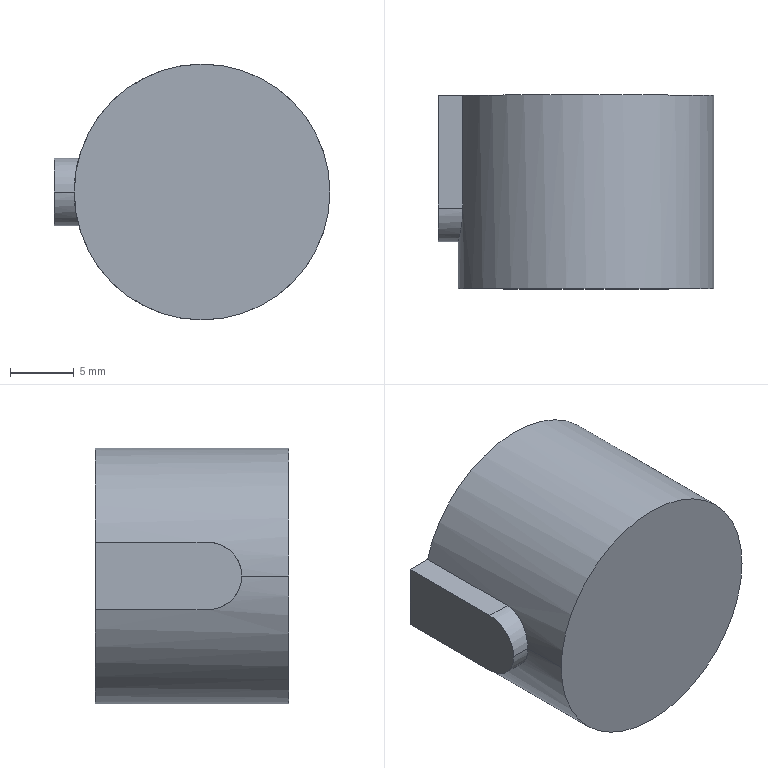Part | SolidWorks | features BaseBody 1 | 1 solid | 9 faces | box 21.648 x 15.198 x 20.064 mm | volume 4903 mm3 | plane 5 | cylinder 4 | commonest cylinder face diameters 5.28 x2 20.064 x2
STEP:
#1=CARTESIAN_POINT('',(-2122.918,1097.894,-1577.624));
#2=VERTEX_POINT('',#1);
#3=CARTESIAN_POINT('',(-2122.918,1082.696,-1577.624));
#4=VERTEX_POINT('',#3);
#5=CARTESIAN_POINT('',(-2122.918,1097.894,-1577.624));
#6=DIRECTION('',(0.,-1.,0.));
#7=VECTOR('',#6,1000.);
#8=LINE('',#5,#7);
#9=EDGE_CURVE('',#2,#4,#8,.T.);
#10=ORIENTED_EDGE('',*,*,#9,.F.);
#11=CARTESIAN_POINT('',(-2142.628,1097.894,-1574.984));
#12=VERTEX_POINT('',#11);
#13=CARTESIAN_POINT('',(-2132.95,1097.894,-1577.624));
#14=DIRECTION('',(0.,-1.,0.));
#15=DIRECTION('',(1.,0.,0.));
#16=AXIS2_PLACEMENT_3D('',#13,#14,#15);
#17=CIRCLE('',#16,10.032);
#18=EDGE_CURVE('',#2,#12,#17,.T.);
#19=ORIENTED_EDGE('',*,*,#18,.T.);
#20=CARTESIAN_POINT('',(-2142.628,1089.032,-1574.984));
#21=VERTEX_POINT('',#20);
#22=CARTESIAN_POINT('',(-2142.628,1089.032,-1574.984));
#23=DIRECTION('',(0.,1.,0.));
#24=VECTOR('',#23,1000.);
#25=LINE('',#22,#24);
#26=EDGE_CURVE('',#21,#12,#25,.T.);
#27=ORIENTED_EDGE('',*,*,#26,.F.);
#28=CARTESIAN_POINT('',(-2142.982,1086.392,-1577.624));
#29=VERTEX_POINT('',#28);
#30=CARTESIAN_POINT('',(-2142.982,1086.392,-1577.624));
#31=CARTESIAN_POINT('',(-2142.982,1086.392,-1577.461));
#32=CARTESIAN_POINT('',(-2142.978,1086.407,-1577.293));
#33=CARTESIAN_POINT('',(-2142.965,1086.456,-1577.038));
#34=CARTESIAN_POINT('',(-2142.959,1086.477,-1576.952));
#35=CARTESIAN_POINT('',(-2142.95,1086.516,-1576.824));
#36=CARTESIAN_POINT('',(-2142.945,1086.537,-1576.761));
#37=CARTESIAN_POINT('',(-2142.938,1086.564,-1576.686));
#38=CARTESIAN_POINT('',(-2142.935,1086.577,-1576.654));
#39=CARTESIAN_POINT('',(-2142.933,1086.585,-1576.633));
#40=CARTESIAN_POINT('',(-2142.931,1086.59,-1576.621));
#41=CARTESIAN_POINT('',(-2142.923,1086.624,-1576.54));
#42=CARTESIAN_POINT('',(-2142.915,1086.659,-1576.465));
#43=CARTESIAN_POINT('',(-2142.9,1086.719,-1576.35));
#44=CARTESIAN_POINT('',(-2142.895,1086.741,-1576.312));
#45=CARTESIAN_POINT('',(-2142.888,1086.776,-1576.254));
#46=CARTESIAN_POINT('',(-2142.884,1086.793,-1576.224));
#47=CARTESIAN_POINT('',(-2142.879,1086.815,-1576.19));
#48=CARTESIAN_POINT('',(-2142.877,1086.825,-1576.176));
#49=CARTESIAN_POINT('',(-2142.875,1086.831,-1576.166));
#50=CARTESIAN_POINT('',(-2142.874,1086.836,-1576.159));
#51=CARTESIAN_POINT('',(-2142.866,1086.871,-1576.106));
#52=CARTESIAN_POINT('',(-2142.857,1086.914,-1576.046));
#53=CARTESIAN_POINT('',(-2142.84,1086.994,-1575.945));
#54=CARTESIAN_POINT('',(-2142.834,1087.024,-1575.91));
#55=CARTESIAN_POINT('',(-2142.824,1087.073,-1575.854));
#56=CARTESIAN_POINT('',(-2142.821,1087.09,-1575.835));
#57=CARTESIAN_POINT('',(-2142.814,1087.127,-1575.797));
#58=CARTESIAN_POINT('',(-2142.81,1087.144,-1575.778));
#59=CARTESIAN_POINT('',(-2142.791,1087.249,-1575.674));
#60=CARTESIAN_POINT('',(-2142.777,1087.326,-1575.608));
#61=CARTESIAN_POINT('',(-2142.76,1087.427,-1575.528));
#62=CARTESIAN_POINT('',(-2142.755,1087.459,-1575.504));
#63=CARTESIAN_POINT('',(-2142.748,1087.501,-1575.473));
#64=CARTESIAN_POINT('',(-2142.745,1087.522,-1575.459));
#65=CARTESIAN_POINT('',(-2142.742,1087.543,-1575.444));
#66=CARTESIAN_POINT('',(-2142.74,1087.554,-1575.437));
#67=CARTESIAN_POINT('',(-2142.74,1087.558,-1575.434));
#68=CARTESIAN_POINT('',(-2142.739,1087.561,-1575.432));
#69=CARTESIAN_POINT('',(-2142.739,1087.561,-1575.432));
#70=CARTESIAN_POINT('',(-2142.727,1087.643,-1575.377));
#71=CARTESIAN_POINT('',(-2142.716,1087.721,-1575.331));
#72=CARTESIAN_POINT('',(-2142.702,1087.835,-1575.271));
#73=CARTESIAN_POINT('',(-2142.697,1087.873,-1575.252));
#74=CARTESIAN_POINT('',(-2142.691,1087.929,-1575.226));
#75=CARTESIAN_POINT('',(-2142.688,1087.956,-1575.213));
#76=CARTESIAN_POINT('',(-2142.685,1087.984,-1575.201));
#77=CARTESIAN_POINT('',(-2142.683,1088.002,-1575.194));
#78=CARTESIAN_POINT('',(-2142.682,1088.009,-1575.191));
#79=CARTESIAN_POINT('',(-2142.646,1088.36,-1575.045));
#80=CARTESIAN_POINT('',(-2142.628,1088.707,-1574.984));
#81=CARTESIAN_POINT('',(-2142.628,1089.032,-1574.984));
#82=B_SPLINE_CURVE_WITH_KNOTS('',3,(#30,#31,#32,#33,#34,#35,#36,#37,#38,#39,#40,#41,#42,#43,#44,#45,#46,#47,#48,#49,#50,#51,#52,#53,#54,#55,#56,#57,#58,#59,#60,#61,#62,#63,#64,#65,#66,#67,#68,#69,#70,#71,#72,#73,#74,#75,#76,#77,#78,#79,#80,#81),.UNSPECIFIED.,.F.,.F.,(4,2,2,1,1,2,2,2,2,1,1,2,2,2,2,2,2,2,2,1,1,1,2,2,2,2,1,2,2,4),(0.,0.125,0.1875,0.2187,0.2344,0.2422,0.25,0.3125,0.3437,0.3594,0.3672,0.3711,0.375,0.4375,0.4687,0.4844,0.5,0.5625,0.5937,0.6094,0.6172,0.6211,0.623,0.625,0.6875,0.7187,0.7344,0.7422,0.75,1.),.UNSPECIFIED.);
#83=EDGE_CURVE('',#29,#21,#82,.T.);
#84=ORIENTED_EDGE('',*,*,#83,.F.);
#85=CARTESIAN_POINT('',(-2142.982,1082.696,-1577.624));
#86=VERTEX_POINT('',#85);
#87=CARTESIAN_POINT('',(-2142.982,1086.392,-1577.624));
#88=DIRECTION('',(0.,-1.,0.));
#89=VECTOR('',#88,1000.);
#90=LINE('',#87,#89);
#91=EDGE_CURVE('',#29,#86,#90,.T.);
#92=ORIENTED_EDGE('',*,*,#91,.T.);
#93=CARTESIAN_POINT('',(-2132.95,1082.696,-1577.624));
#94=DIRECTION('',(0.,-1.,0.));
#95=DIRECTION('',(1.,0.,0.));
#96=AXIS2_PLACEMENT_3D('',#93,#94,#95);
#97=CIRCLE('',#96,10.032);
#98=EDGE_CURVE('',#4,#86,#97,.T.);
#99=ORIENTED_EDGE('',*,*,#98,.F.);
#100=EDGE_LOOP('',(#10,#19,#27,#84,#92,#99));
#101=FACE_OUTER_BOUND('',#100,.T.);
#102=CARTESIAN_POINT('',(-2132.95,1080.69,-1577.624));
#103=DIRECTION('',(0.,-1.,0.));
#104=DIRECTION('',(0.9962,0.,-0.08716));
#105=AXIS2_PLACEMENT_3D('',#102,#103,#104);
#106=CYLINDRICAL_SURFACE('',#105,10.032);
#107=ADVANCED_FACE('',(#101),#106,.T.);
#108=CARTESIAN_POINT('',(-2144.566,1097.894,-1580.264));
#109=VERTEX_POINT('',#108);
#110=CARTESIAN_POINT('',(-2144.566,1097.894,-1574.984));
#111=VERTEX_POINT('',#110);
#112=CARTESIAN_POINT('',(-2144.566,1097.894,-1580.264));
#113=DIRECTION('',(0.,0.,1.));
#114=VECTOR('',#113,1000.);
#115=LINE('',#112,#114);
#116=EDGE_CURVE('',#109,#111,#115,.T.);
#117=ORIENTED_EDGE('',*,*,#116,.F.);
#118=CARTESIAN_POINT('',(-2144.566,1089.032,-1580.264));
#119=VERTEX_POINT('',#118);
#120=CARTESIAN_POINT('',(-2144.566,1097.894,-1580.264));
#121=DIRECTION('',(0.,-1.,0.));
#122=VECTOR('',#121,1000.);
#123=LINE('',#120,#122);
#124=EDGE_CURVE('',#109,#119,#123,.T.);
#125=ORIENTED_EDGE('',*,*,#124,.T.);
#126=CARTESIAN_POINT('',(-2144.566,1086.392,-1577.624));
#127=VERTEX_POINT('',#126);
#128=CARTESIAN_POINT('',(-2144.566,1089.032,-1577.624));
#129=DIRECTION('',(-1.,0.,0.));
#130=DIRECTION('',(0.,0.,-1.));
#131=AXIS2_PLACEMENT_3D('',#128,#129,#130);
#132=CIRCLE('',#131,2.64);
#133=EDGE_CURVE('',#119,#127,#132,.T.);
#134=ORIENTED_EDGE('',*,*,#133,.T.);
#135=CARTESIAN_POINT('',(-2144.566,1089.032,-1574.984));
#136=VERTEX_POINT('',#135);
#137=CARTESIAN_POINT('',(-2144.566,1089.032,-1577.624));
#138=DIRECTION('',(-1.,0.,0.));
#139=DIRECTION('',(0.,-1.,0.));
#140=AXIS2_PLACEMENT_3D('',#137,#138,#139);
#141=CIRCLE('',#140,2.64);
#142=EDGE_CURVE('',#127,#136,#141,.T.);
#143=ORIENTED_EDGE('',*,*,#142,.T.);
#144=CARTESIAN_POINT('',(-2144.566,1089.032,-1574.984));
#145=DIRECTION('',(0.,1.,0.));
#146=VECTOR('',#145,1000.);
#147=LINE('',#144,#146);
#148=EDGE_CURVE('',#136,#111,#147,.T.);
#149=ORIENTED_EDGE('',*,*,#148,.T.);
#150=EDGE_LOOP('',(#117,#125,#134,#143,#149));
#151=FACE_OUTER_BOUND('',#150,.T.);
#152=CARTESIAN_POINT('',(-2144.566,1084.729,-1573.321));
#153=DIRECTION('',(-1.,0.,0.));
#154=DIRECTION('',(0.,0.,1.));
#155=AXIS2_PLACEMENT_3D('',#152,#153,#154);
#156=PLANE('',#155);
#157=ADVANCED_FACE('',(#151),#156,.T.);
#158=ORIENTED_EDGE('',*,*,#142,.F.);
#159=CARTESIAN_POINT('',(-2144.566,1086.392,-1577.624));
#160=DIRECTION('',(1.,0.,0.));
#161=VECTOR('',#160,1000.);
#162=LINE('',#159,#161);
#163=EDGE_CURVE('',#127,#29,#162,.T.);
#164=ORIENTED_EDGE('',*,*,#163,.T.);
#165=ORIENTED_EDGE('',*,*,#83,.T.);
#166=CARTESIAN_POINT('',(-2142.628,1089.032,-1574.984));
#167=DIRECTION('',(-1.,-0.000000001,0.));
#168=VECTOR('',#167,1000.);
#169=LINE('',#166,#168);
#170=EDGE_CURVE('',#21,#136,#169,.T.);
#171=ORIENTED_EDGE('',*,*,#170,.T.);
#172=EDGE_LOOP('',(#158,#164,#165,#171));
#173=FACE_OUTER_BOUND('',#172,.T.);
#174=CARTESIAN_POINT('',(-2142.531,1089.032,-1577.624));
#175=DIRECTION('',(1.,0.,0.));
#176=DIRECTION('',(0.,0.08716,0.9962));
#177=AXIS2_PLACEMENT_3D('',#174,#175,#176);
#178=CYLINDRICAL_SURFACE('',#177,2.64);
#179=ADVANCED_FACE('',(#173),#178,.T.);
#180=ORIENTED_EDGE('',*,*,#26,.T.);
#181=CARTESIAN_POINT('',(-2144.566,1097.894,-1574.984));
#182=DIRECTION('',(1.,0.,0.));
#183=VECTOR('',#182,1000.);
#184=LINE('',#181,#183);
#185=EDGE_CURVE('',#111,#12,#184,.T.);
#186=ORIENTED_EDGE('',*,*,#185,.F.);
#187=ORIENTED_EDGE('',*,*,#148,.F.);
#188=ORIENTED_EDGE('',*,*,#170,.F.);
#189=EDGE_LOOP('',(#180,#186,#187,#188));
#190=FACE_OUTER_BOUND('',#189,.T.);
#191=CARTESIAN_POINT('',(-2141.229,1118.415,-1574.984));
#192=DIRECTION('',(0.,0.,1.));
#193=DIRECTION('',(1.,0.,0.));
#194=AXIS2_PLACEMENT_3D('',#191,#192,#193);
#195=PLANE('',#194);
#196=ADVANCED_FACE('',(#190),#195,.T.);
#197=CARTESIAN_POINT('',(-2142.628,1097.894,-1580.264));
#198=VERTEX_POINT('',#197);
#199=CARTESIAN_POINT('',(-2142.628,1097.894,-1580.264));
#200=DIRECTION('',(-1.,0.,0.));
#201=VECTOR('',#200,1000.);
#202=LINE('',#199,#201);
#203=EDGE_CURVE('',#198,#109,#202,.T.);
#204=ORIENTED_EDGE('',*,*,#203,.F.);
#205=CARTESIAN_POINT('',(-2142.628,1089.032,-1580.264));
#206=VERTEX_POINT('',#205);
#207=CARTESIAN_POINT('',(-2142.628,1097.894,-1580.264));
#208=DIRECTION('',(0.,-1.,0.));
#209=VECTOR('',#208,1000.);
#210=LINE('',#207,#209);
#211=EDGE_CURVE('',#198,#206,#210,.T.);
#212=ORIENTED_EDGE('',*,*,#211,.T.);
#213=CARTESIAN_POINT('',(-2142.628,1089.032,-1580.264));
#214=DIRECTION('',(-1.,0.,0.));
#215=VECTOR('',#214,1000.);
#216=LINE('',#213,#215);
#217=EDGE_CURVE('',#206,#119,#216,.T.);
#218=ORIENTED_EDGE('',*,*,#217,.T.);
#219=ORIENTED_EDGE('',*,*,#124,.F.);
#220=EDGE_LOOP('',(#204,#212,#218,#219));
#221=FACE_OUTER_BOUND('',#220,.T.);
#222=CARTESIAN_POINT('',(-2145.965,1118.415,-1580.264));
#223=DIRECTION('',(0.,0.,-1.));
#224=DIRECTION('',(0.,-1.,0.));
#225=AXIS2_PLACEMENT_3D('',#222,#223,#224);
#226=PLANE('',#225);
#227=ADVANCED_FACE('',(#221),#226,.T.);
#228=CARTESIAN_POINT('',(-2132.95,1082.696,-1577.624));
#229=DIRECTION('',(0.,-1.,0.));
#230=DIRECTION('',(-1.,0.,0.));
#231=AXIS2_PLACEMENT_3D('',#228,#229,#230);
#232=CIRCLE('',#231,10.032);
#233=EDGE_CURVE('',#86,#4,#232,.T.);
#234=ORIENTED_EDGE('',*,*,#233,.T.);
#235=ORIENTED_EDGE('',*,*,#98,.T.);
#236=EDGE_LOOP('',(#234,#235));
#237=FACE_OUTER_BOUND('',#236,.T.);
#238=CARTESIAN_POINT('',(-2143.985,1082.696,-1588.66));
#239=DIRECTION('',(0.,-1.,0.));
#240=DIRECTION('',(0.,0.,-1.));
#241=AXIS2_PLACEMENT_3D('',#238,#239,#240);
#242=PLANE('',#241);
#243=ADVANCED_FACE('',(#237),#242,.T.);
#244=ORIENTED_EDGE('',*,*,#163,.F.);
#245=ORIENTED_EDGE('',*,*,#133,.F.);
#246=ORIENTED_EDGE('',*,*,#217,.F.);
#247=CARTESIAN_POINT('',(-2142.628,1089.032,-1580.264));
#248=CARTESIAN_POINT('',(-2142.628,1088.87,-1580.264));
#249=CARTESIAN_POINT('',(-2142.632,1088.702,-1580.249));
#250=CARTESIAN_POINT('',(-2142.646,1088.447,-1580.2));
#251=CARTESIAN_POINT('',(-2142.651,1088.361,-1580.179));
#252=CARTESIAN_POINT('',(-2142.661,1088.233,-1580.141));
#253=CARTESIAN_POINT('',(-2142.666,1088.169,-1580.12));
#254=CARTESIAN_POINT('',(-2142.673,1088.094,-1580.092));
#255=CARTESIAN_POINT('',(-2142.677,1088.062,-1580.08));
#256=CARTESIAN_POINT('',(-2142.679,1088.041,-1580.071));
#257=CARTESIAN_POINT('',(-2142.68,1088.029,-1580.066));
#258=CARTESIAN_POINT('',(-2142.688,1087.948,-1580.033));
#259=CARTESIAN_POINT('',(-2142.697,1087.874,-1579.998));
#260=CARTESIAN_POINT('',(-2142.711,1087.759,-1579.938));
#261=CARTESIAN_POINT('',(-2142.716,1087.72,-1579.916));
#262=CARTESIAN_POINT('',(-2142.725,1087.662,-1579.881));
#263=CARTESIAN_POINT('',(-2142.729,1087.633,-1579.863));
#264=CARTESIAN_POINT('',(-2142.734,1087.598,-1579.841));
#265=CARTESIAN_POINT('',(-2142.736,1087.581,-1579.83));
#266=CARTESIAN_POINT('',(-2142.737,1087.574,-1579.825));
#267=CARTESIAN_POINT('',(-2142.738,1087.569,-1579.822));
#268=CARTESIAN_POINT('',(-2142.739,1087.565,-1579.819));
#269=CARTESIAN_POINT('',(-2142.746,1087.519,-1579.788));
#270=CARTESIAN_POINT('',(-2142.755,1087.461,-1579.748));
#271=CARTESIAN_POINT('',(-2142.771,1087.36,-1579.668));
#272=CARTESIAN_POINT('',(-2142.778,1087.324,-1579.638));
#273=CARTESIAN_POINT('',(-2142.788,1087.266,-1579.587));
#274=CARTESIAN_POINT('',(-2142.791,1087.247,-1579.57));
#275=CARTESIAN_POINT('',(-2142.799,1087.207,-1579.532));
#276=CARTESIAN_POINT('',(-2142.803,1087.185,-1579.511));
#277=CARTESIAN_POINT('',(-2142.821,1087.086,-1579.412));
#278=CARTESIAN_POINT('',(-2142.835,1087.021,-1579.337));
#279=CARTESIAN_POINT('',(-2142.851,1086.941,-1579.236));
#280=CARTESIAN_POINT('',(-2142.856,1086.917,-1579.204));
#281=CARTESIAN_POINT('',(-2142.863,1086.884,-1579.16));
#282=CARTESIAN_POINT('',(-2142.867,1086.869,-1579.139));
#283=CARTESIAN_POINT('',(-2142.87,1086.853,-1579.115));
#284=CARTESIAN_POINT('',(-2142.872,1086.846,-1579.105));
#285=CARTESIAN_POINT('',(-2142.873,1086.842,-1579.099));
#286=CARTESIAN_POINT('',(-2142.873,1086.841,-1579.098));
#287=CARTESIAN_POINT('',(-2142.885,1086.786,-1579.015));
#288=CARTESIAN_POINT('',(-2142.896,1086.74,-1578.937));
#289=CARTESIAN_POINT('',(-2142.91,1086.679,-1578.822));
#290=CARTESIAN_POINT('',(-2142.914,1086.66,-1578.784));
#291=CARTESIAN_POINT('',(-2142.921,1086.634,-1578.728));
#292=CARTESIAN_POINT('',(-2142.924,1086.621,-1578.701));
#293=CARTESIAN_POINT('',(-2142.927,1086.609,-1578.673));
#294=CARTESIAN_POINT('',(-2142.929,1086.601,-1578.655));
#295=CARTESIAN_POINT('',(-2142.929,1086.598,-1578.647));
#296=CARTESIAN_POINT('',(-2142.965,1086.453,-1578.299));
#297=CARTESIAN_POINT('',(-2142.982,1086.392,-1577.951));
#298=CARTESIAN_POINT('',(-2142.982,1086.392,-1577.624));
#299=B_SPLINE_CURVE_WITH_KNOTS('',3,(#247,#248,#249,#250,#251,#252,#253,#254,#255,#256,#257,#258,#259,#260,#261,#262,#263,#264,#265,#266,#267,#268,#269,#270,#271,#272,#273,#274,#275,#276,#277,#278,#279,#280,#281,#282,#283,#284,#285,#286,#287,#288,#289,#290,#291,#292,#293,#294,#295,#296,#297,#298),.UNSPECIFIED.,.F.,.F.,(4,2,2,1,1,2,2,2,2,1,1,1,2,2,2,2,2,2,2,2,1,1,2,2,2,2,1,2,2,4),(0.,0.125,0.1875,0.2187,0.2344,0.2422,0.25,0.3125,0.3437,0.3594,0.3672,0.3711,0.373,0.375,0.4375,0.4687,0.4844,0.5,0.5625,0.5937,0.6094,0.6172,0.6211,0.625,0.6875,0.7187,0.7344,0.7422,0.75,1.),.UNSPECIFIED.);
#300=EDGE_CURVE('',#206,#29,#299,.T.);
#301=ORIENTED_EDGE('',*,*,#300,.T.);
#302=EDGE_LOOP('',(#244,#245,#246,#301));
#303=FACE_OUTER_BOUND('',#302,.T.);
#304=CARTESIAN_POINT('',(-2142.531,1089.032,-1577.624));
#305=DIRECTION('',(1.,0.,0.));
#306=DIRECTION('',(0.,-0.9962,0.08716));
#307=AXIS2_PLACEMENT_3D('',#304,#305,#306);
#308=CYLINDRICAL_SURFACE('',#307,2.64);
#309=ADVANCED_FACE('',(#303),#308,.T.);
#310=CARTESIAN_POINT('',(-2132.95,1097.894,-1577.624));
#311=DIRECTION('',(0.,-1.,0.));
#312=DIRECTION('',(-0.9648,0.,-0.2632));
#313=AXIS2_PLACEMENT_3D('',#310,#311,#312);
#314=CIRCLE('',#313,10.032);
#315=EDGE_CURVE('',#198,#2,#314,.T.);
#316=ORIENTED_EDGE('',*,*,#315,.T.);
#317=ORIENTED_EDGE('',*,*,#9,.T.);
#318=ORIENTED_EDGE('',*,*,#233,.F.);
#319=ORIENTED_EDGE('',*,*,#91,.F.);
#320=ORIENTED_EDGE('',*,*,#300,.F.);
#321=ORIENTED_EDGE('',*,*,#211,.F.);
#322=EDGE_LOOP('',(#316,#317,#318,#319,#320,#321));
#323=FACE_OUTER_BOUND('',#322,.T.);
#324=CARTESIAN_POINT('',(-2132.95,1080.69,-1577.624));
#325=DIRECTION('',(0.,-1.,0.));
#326=DIRECTION('',(-0.9962,0.,0.08716));
#327=AXIS2_PLACEMENT_3D('',#324,#325,#326);
#328=CYLINDRICAL_SURFACE('',#327,10.032);
#329=ADVANCED_FACE('',(#323),#328,.T.);
#330=ORIENTED_EDGE('',*,*,#315,.F.);
#331=ORIENTED_EDGE('',*,*,#203,.T.);
#332=ORIENTED_EDGE('',*,*,#116,.T.);
#333=ORIENTED_EDGE('',*,*,#185,.T.);
#334=ORIENTED_EDGE('',*,*,#18,.F.);
#335=EDGE_LOOP('',(#330,#331,#332,#333,#334));
#336=FACE_OUTER_BOUND('',#335,.T.);
#337=CARTESIAN_POINT('',(-2200.45,1097.894,-1510.124));
#338=DIRECTION('',(0.,1.,0.));
#339=DIRECTION('',(1.,0.,0.));
#340=AXIS2_PLACEMENT_3D('',#337,#338,#339);
#341=PLANE('',#340);
#342=ADVANCED_FACE('',(#336),#341,.T.);
#343=CLOSED_SHELL('',(#107,#157,#179,#196,#227,#243,#309,#329,#342));
#344=MANIFOLD_SOLID_BREP('',#343);
#345=CARTESIAN_POINT('',(0.,0.,0.));
#346=DIRECTION('',(0.,0.,1.));
#347=DIRECTION('',(1.,0.,0.));
#348=AXIS2_PLACEMENT_3D('',#345,#346,#347);
#349=(LENGTH_UNIT()NAMED_UNIT(*)SI_UNIT(.MILLI.,.METRE.));
#350=UNCERTAINTY_MEASURE_WITH_UNIT(LENGTH_MEASURE(0.00001),#349,'','');
#351=(NAMED_UNIT(*)PLANE_ANGLE_UNIT()SI_UNIT($,.RADIAN.));
#352=(NAMED_UNIT(*)SI_UNIT($,.STERADIAN.)SOLID_ANGLE_UNIT());
#353=(GEOMETRIC_REPRESENTATION_CONTEXT(3)GLOBAL_UNCERTAINTY_ASSIGNED_CONTEXT((#350))GLOBAL_UNIT_ASSIGNED_CONTEXT((#349,#351,#352))REPRESENTATION_CONTEXT('',''));
#354=ADVANCED_BREP_SHAPE_REPRESENTATION('',(#344,#348),#353);